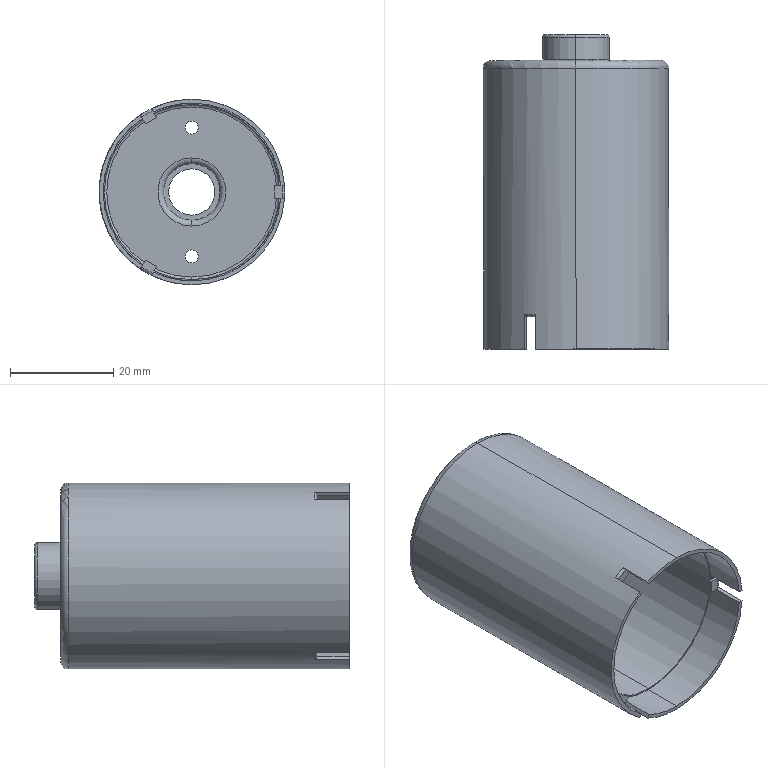Part | SolidWorks | features BaseBody 1 | 1 solid | 60 faces | box 36.046 x 61.023 x 36 mm | volume 6822 mm3 | plane 29 | cylinder 16 | torus 15 | commonest cylinder face diameters 2.5 x4 9 x2 12 x2 13 x2 34 x2 34.5 x2